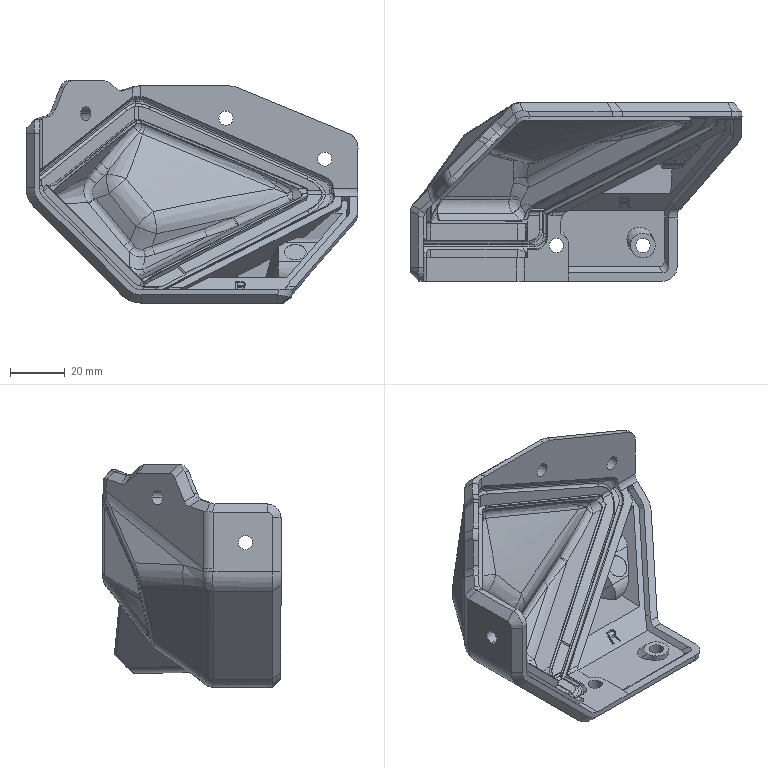Part | SolidWorks | features BaseBody 1 | 1 solid | 534 faces | box 121.203 x 65.012 x 81.18 mm | volume 61881 mm3 | spline 189 | plane 168 | cylinder 160 | sphere 6 | cone 6 | torus 5 | commonest cylinder face diameters 0.6 x16 0.4 x15 4 x15 5.2 x13 10 x13 8 x12